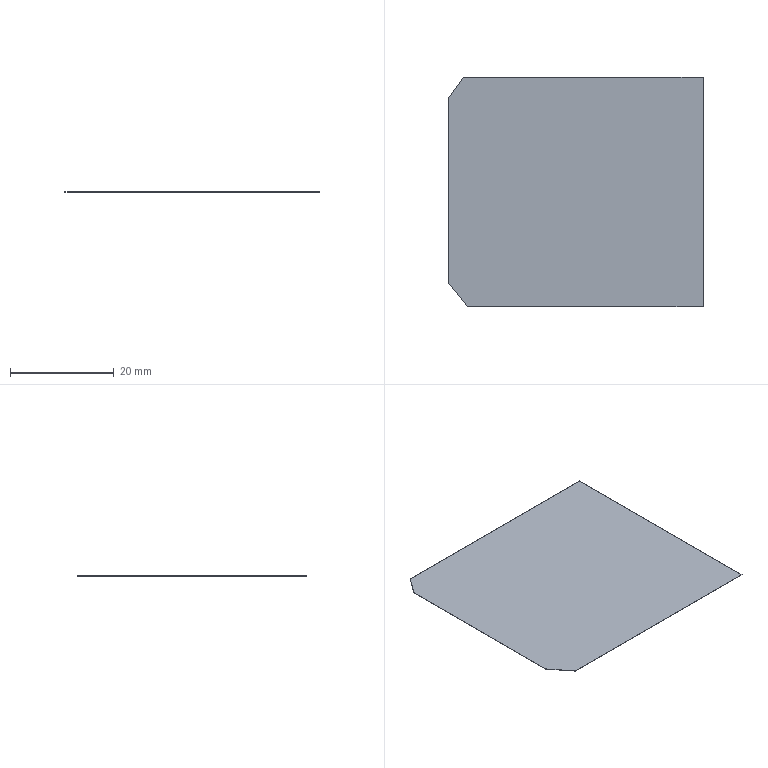Part | NX | features DATUM_CSYS 2, EXTRUDE 1, SKETCH 1 | 1 solid | 8 faces | box 49.09 x 44.4 x 0.05 mm | volume 108.301 mm3 | plane 8
STEP:
#1=CARTESIAN_POINT('',(0.,40.48,0.));
#2=VERTEX_POINT('',#1);
#3=CARTESIAN_POINT('',(0.,4.52,0.));
#4=VERTEX_POINT('',#3);
#5=CARTESIAN_POINT('',(0.,40.48,0.));
#6=DIRECTION('',(0.,-1.,0.));
#7=VECTOR('',#6,1000.);
#8=LINE('',#5,#7);
#9=EDGE_CURVE('',#2,#4,#8,.T.);
#10=ORIENTED_EDGE('',*,*,#9,.T.);
#11=CARTESIAN_POINT('',(0.,4.52,0.05));
#12=VERTEX_POINT('',#11);
#13=CARTESIAN_POINT('',(0.,4.52,0.05));
#14=DIRECTION('',(0.,0.,-1.));
#15=VECTOR('',#14,1000.);
#16=LINE('',#13,#15);
#17=EDGE_CURVE('',#12,#4,#16,.T.);
#18=ORIENTED_EDGE('',*,*,#17,.F.);
#19=CARTESIAN_POINT('',(0.,40.48,0.05));
#20=VERTEX_POINT('',#19);
#21=CARTESIAN_POINT('',(0.,40.48,0.05));
#22=DIRECTION('',(0.,-1.,0.));
#23=VECTOR('',#22,1000.);
#24=LINE('',#21,#23);
#25=EDGE_CURVE('',#20,#12,#24,.T.);
#26=ORIENTED_EDGE('',*,*,#25,.F.);
#27=CARTESIAN_POINT('',(0.,40.48,0.05));
#28=DIRECTION('',(0.,0.,-1.));
#29=VECTOR('',#28,1000.);
#30=LINE('',#27,#29);
#31=EDGE_CURVE('',#20,#2,#30,.T.);
#32=ORIENTED_EDGE('',*,*,#31,.T.);
#33=EDGE_LOOP('',(#10,#18,#26,#32));
#34=FACE_BOUND('',#33,.T.);
#35=CARTESIAN_POINT('',(0.,40.48,0.05));
#36=DIRECTION('',(1.,0.,0.));
#37=DIRECTION('',(0.,0.,-1.));
#38=AXIS2_PLACEMENT_3D('',#35,#36,#37);
#39=PLANE('',#38);
#40=ADVANCED_FACE('',(#34),#39,.F.);
#41=CARTESIAN_POINT('',(3.59,0.,0.));
#42=VERTEX_POINT('',#41);
#43=CARTESIAN_POINT('',(0.,4.52,0.));
#44=DIRECTION('',(0.6219,-0.7831,0.));
#45=VECTOR('',#44,1000.);
#46=LINE('',#43,#45);
#47=EDGE_CURVE('',#4,#42,#46,.T.);
#48=ORIENTED_EDGE('',*,*,#47,.T.);
#49=CARTESIAN_POINT('',(3.59,0.,0.05));
#50=VERTEX_POINT('',#49);
#51=CARTESIAN_POINT('',(3.59,0.,0.05));
#52=DIRECTION('',(0.,0.,-1.));
#53=VECTOR('',#52,1000.);
#54=LINE('',#51,#53);
#55=EDGE_CURVE('',#50,#42,#54,.T.);
#56=ORIENTED_EDGE('',*,*,#55,.F.);
#57=CARTESIAN_POINT('',(0.,4.52,0.05));
#58=DIRECTION('',(0.6219,-0.7831,0.));
#59=VECTOR('',#58,1000.);
#60=LINE('',#57,#59);
#61=EDGE_CURVE('',#12,#50,#60,.T.);
#62=ORIENTED_EDGE('',*,*,#61,.F.);
#63=ORIENTED_EDGE('',*,*,#17,.T.);
#64=EDGE_LOOP('',(#48,#56,#62,#63));
#65=FACE_BOUND('',#64,.T.);
#66=CARTESIAN_POINT('',(0.,4.52,0.05));
#67=DIRECTION('',(0.7831,0.6219,0.));
#68=DIRECTION('',(-0.6219,0.7831,0.));
#69=AXIS2_PLACEMENT_3D('',#66,#67,#68);
#70=PLANE('',#69);
#71=ADVANCED_FACE('',(#65),#70,.F.);
#72=CARTESIAN_POINT('',(49.09,0.,0.));
#73=VERTEX_POINT('',#72);
#74=CARTESIAN_POINT('',(3.59,0.,0.));
#75=DIRECTION('',(1.,0.,0.));
#76=VECTOR('',#75,1000.);
#77=LINE('',#74,#76);
#78=EDGE_CURVE('',#42,#73,#77,.T.);
#79=ORIENTED_EDGE('',*,*,#78,.T.);
#80=CARTESIAN_POINT('',(49.09,0.,0.05));
#81=VERTEX_POINT('',#80);
#82=CARTESIAN_POINT('',(49.09,0.,0.05));
#83=DIRECTION('',(0.,0.,-1.));
#84=VECTOR('',#83,1000.);
#85=LINE('',#82,#84);
#86=EDGE_CURVE('',#81,#73,#85,.T.);
#87=ORIENTED_EDGE('',*,*,#86,.F.);
#88=CARTESIAN_POINT('',(3.59,0.,0.05));
#89=DIRECTION('',(1.,0.,0.));
#90=VECTOR('',#89,1000.);
#91=LINE('',#88,#90);
#92=EDGE_CURVE('',#50,#81,#91,.T.);
#93=ORIENTED_EDGE('',*,*,#92,.F.);
#94=ORIENTED_EDGE('',*,*,#55,.T.);
#95=EDGE_LOOP('',(#79,#87,#93,#94));
#96=FACE_BOUND('',#95,.T.);
#97=CARTESIAN_POINT('',(3.59,0.,0.05));
#98=DIRECTION('',(0.,1.,0.));
#99=DIRECTION('',(-1.,0.,0.));
#100=AXIS2_PLACEMENT_3D('',#97,#98,#99);
#101=PLANE('',#100);
#102=ADVANCED_FACE('',(#96),#101,.F.);
#103=CARTESIAN_POINT('',(49.09,44.4,0.));
#104=VERTEX_POINT('',#103);
#105=CARTESIAN_POINT('',(49.09,0.,0.));
#106=DIRECTION('',(0.,1.,0.));
#107=VECTOR('',#106,1000.);
#108=LINE('',#105,#107);
#109=EDGE_CURVE('',#73,#104,#108,.T.);
#110=ORIENTED_EDGE('',*,*,#109,.T.);
#111=CARTESIAN_POINT('',(49.09,44.4,0.05));
#112=VERTEX_POINT('',#111);
#113=CARTESIAN_POINT('',(49.09,44.4,0.05));
#114=DIRECTION('',(0.,0.,-1.));
#115=VECTOR('',#114,1000.);
#116=LINE('',#113,#115);
#117=EDGE_CURVE('',#112,#104,#116,.T.);
#118=ORIENTED_EDGE('',*,*,#117,.F.);
#119=CARTESIAN_POINT('',(49.09,0.,0.05));
#120=DIRECTION('',(0.,1.,0.));
#121=VECTOR('',#120,1000.);
#122=LINE('',#119,#121);
#123=EDGE_CURVE('',#81,#112,#122,.T.);
#124=ORIENTED_EDGE('',*,*,#123,.F.);
#125=ORIENTED_EDGE('',*,*,#86,.T.);
#126=EDGE_LOOP('',(#110,#118,#124,#125));
#127=FACE_BOUND('',#126,.T.);
#128=CARTESIAN_POINT('',(49.09,0.,0.05));
#129=DIRECTION('',(-1.,0.,0.));
#130=DIRECTION('',(0.,0.,1.));
#131=AXIS2_PLACEMENT_3D('',#128,#129,#130);
#132=PLANE('',#131);
#133=ADVANCED_FACE('',(#127),#132,.F.);
#134=CARTESIAN_POINT('',(2.79,44.4,0.));
#135=VERTEX_POINT('',#134);
#136=CARTESIAN_POINT('',(49.09,44.4,0.));
#137=DIRECTION('',(-1.,0.,0.));
#138=VECTOR('',#137,1000.);
#139=LINE('',#136,#138);
#140=EDGE_CURVE('',#104,#135,#139,.T.);
#141=ORIENTED_EDGE('',*,*,#140,.T.);
#142=CARTESIAN_POINT('',(2.79,44.4,0.05));
#143=VERTEX_POINT('',#142);
#144=CARTESIAN_POINT('',(2.79,44.4,0.05));
#145=DIRECTION('',(0.,0.,-1.));
#146=VECTOR('',#145,1000.);
#147=LINE('',#144,#146);
#148=EDGE_CURVE('',#143,#135,#147,.T.);
#149=ORIENTED_EDGE('',*,*,#148,.F.);
#150=CARTESIAN_POINT('',(49.09,44.4,0.05));
#151=DIRECTION('',(-1.,0.,0.));
#152=VECTOR('',#151,1000.);
#153=LINE('',#150,#152);
#154=EDGE_CURVE('',#112,#143,#153,.T.);
#155=ORIENTED_EDGE('',*,*,#154,.F.);
#156=ORIENTED_EDGE('',*,*,#117,.T.);
#157=EDGE_LOOP('',(#141,#149,#155,#156));
#158=FACE_BOUND('',#157,.T.);
#159=CARTESIAN_POINT('',(49.09,44.4,0.05));
#160=DIRECTION('',(0.,-1.,0.));
#161=DIRECTION('',(0.,0.,-1.));
#162=AXIS2_PLACEMENT_3D('',#159,#160,#161);
#163=PLANE('',#162);
#164=ADVANCED_FACE('',(#158),#163,.F.);
#165=CARTESIAN_POINT('',(2.79,44.4,0.));
#166=DIRECTION('',(-0.5799,-0.8147,0.));
#167=VECTOR('',#166,1000.);
#168=LINE('',#165,#167);
#169=EDGE_CURVE('',#135,#2,#168,.T.);
#170=ORIENTED_EDGE('',*,*,#169,.T.);
#171=ORIENTED_EDGE('',*,*,#31,.F.);
#172=CARTESIAN_POINT('',(2.79,44.4,0.05));
#173=DIRECTION('',(-0.5799,-0.8147,0.));
#174=VECTOR('',#173,1000.);
#175=LINE('',#172,#174);
#176=EDGE_CURVE('',#143,#20,#175,.T.);
#177=ORIENTED_EDGE('',*,*,#176,.F.);
#178=ORIENTED_EDGE('',*,*,#148,.T.);
#179=EDGE_LOOP('',(#170,#171,#177,#178));
#180=FACE_BOUND('',#179,.T.);
#181=CARTESIAN_POINT('',(2.79,44.4,0.05));
#182=DIRECTION('',(0.8147,-0.5799,0.));
#183=DIRECTION('',(0.5799,0.8147,0.));
#184=AXIS2_PLACEMENT_3D('',#181,#182,#183);
#185=PLANE('',#184);
#186=ADVANCED_FACE('',(#180),#185,.F.);
#187=ORIENTED_EDGE('',*,*,#25,.T.);
#188=ORIENTED_EDGE('',*,*,#61,.T.);
#189=ORIENTED_EDGE('',*,*,#92,.T.);
#190=ORIENTED_EDGE('',*,*,#123,.T.);
#191=ORIENTED_EDGE('',*,*,#154,.T.);
#192=ORIENTED_EDGE('',*,*,#176,.T.);
#193=EDGE_LOOP('',(#187,#188,#189,#190,#191,#192));
#194=FACE_BOUND('',#193,.T.);
#195=CARTESIAN_POINT('',(0.,0.,0.05));
#196=DIRECTION('',(0.,0.,1.));
#197=DIRECTION('',(1.,0.,0.));
#198=AXIS2_PLACEMENT_3D('',#195,#196,#197);
#199=PLANE('',#198);
#200=ADVANCED_FACE('',(#194),#199,.T.);
#201=ORIENTED_EDGE('',*,*,#9,.F.);
#202=ORIENTED_EDGE('',*,*,#169,.F.);
#203=ORIENTED_EDGE('',*,*,#140,.F.);
#204=ORIENTED_EDGE('',*,*,#109,.F.);
#205=ORIENTED_EDGE('',*,*,#78,.F.);
#206=ORIENTED_EDGE('',*,*,#47,.F.);
#207=EDGE_LOOP('',(#201,#202,#203,#204,#205,#206));
#208=FACE_BOUND('',#207,.T.);
#209=CARTESIAN_POINT('',(0.,0.,0.));
#210=DIRECTION('',(0.,0.,1.));
#211=DIRECTION('',(1.,0.,0.));
#212=AXIS2_PLACEMENT_3D('',#209,#210,#211);
#213=PLANE('',#212);
#214=ADVANCED_FACE('',(#208),#213,.F.);
#215=CLOSED_SHELL('',(#40,#71,#102,#133,#164,#186,#200,#214));
#216=MANIFOLD_SOLID_BREP('',#215);
#217=(LENGTH_UNIT()NAMED_UNIT(*)SI_UNIT(.MILLI.,.METRE.));
#218=UNCERTAINTY_MEASURE_WITH_UNIT(LENGTH_MEASURE(0.00001),#217,'','');
#219=(NAMED_UNIT(*)PLANE_ANGLE_UNIT()SI_UNIT($,.RADIAN.));
#220=(NAMED_UNIT(*)SI_UNIT($,.STERADIAN.)SOLID_ANGLE_UNIT());
#221=(GEOMETRIC_REPRESENTATION_CONTEXT(3)GLOBAL_UNCERTAINTY_ASSIGNED_CONTEXT((#218))GLOBAL_UNIT_ASSIGNED_CONTEXT((#217,#219,#220))REPRESENTATION_CONTEXT('',''));
#222=ADVANCED_BREP_SHAPE_REPRESENTATION('',(#216),#221);